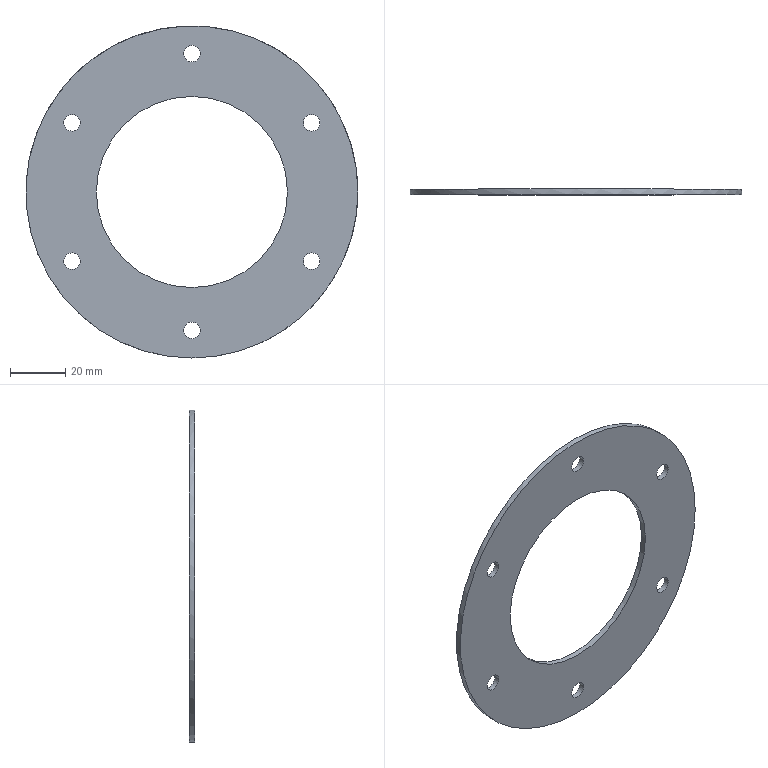Part | NX | features DATUM_CSYS 12, SKETCH 11, HOLE PACKAGE 9, SIMPLE HOLE 9, EXTRACT_DATUM_AXIS 6, EXTRACT_FACE 6, Instance Feature 5, EXTRUDE 4, BLEND 2, DELETE FACE 1, Pattern Feature 1, REPLACE_FACE 1, SWP104 1 | 1 solid | 10 faces | box 120 x 2 x 120 mm | volume 14781 mm3 | cylinder 8 | plane 2 | commonest cylinder face diameters 6 x6 69.097 x1 120 x1
STEP:
#1=CARTESIAN_POINT('',(0.,-9.6,-34.549));
#2=VERTEX_POINT('',#1);
#3=CARTESIAN_POINT('',(0.,-9.6,0.));
#4=DIRECTION('',(0.,-1.,0.));
#5=DIRECTION('',(0.,0.,-1.));
#6=AXIS2_PLACEMENT_3D('',#3,#4,#5);
#7=CIRCLE('',#6,34.549);
#8=EDGE_CURVE('',#2,#2,#7,.F.);
#9=ORIENTED_EDGE('',*,*,#8,.T.);
#10=EDGE_LOOP('',(#9));
#11=FACE_BOUND('',#10,.T.);
#12=CARTESIAN_POINT('',(60.,-9.6,0.));
#13=VERTEX_POINT('',#12);
#14=CARTESIAN_POINT('',(0.,-9.6,0.));
#15=DIRECTION('',(0.,-1.,0.));
#16=DIRECTION('',(1.,0.,0.));
#17=AXIS2_PLACEMENT_3D('',#14,#15,#16);
#18=CIRCLE('',#17,60.);
#19=EDGE_CURVE('',#13,#13,#18,.T.);
#20=ORIENTED_EDGE('',*,*,#19,.T.);
#21=EDGE_LOOP('',(#20));
#22=FACE_BOUND('',#21,.T.);
#23=CARTESIAN_POINT('',(0.,-9.6,53.));
#24=VERTEX_POINT('',#23);
#25=CARTESIAN_POINT('',(0.,-9.6,50.));
#26=DIRECTION('',(0.,1.,0.));
#27=DIRECTION('',(0.,0.,1.));
#28=AXIS2_PLACEMENT_3D('',#25,#26,#27);
#29=CIRCLE('',#28,3.);
#30=EDGE_CURVE('',#24,#24,#29,.T.);
#31=ORIENTED_EDGE('',*,*,#30,.T.);
#32=EDGE_LOOP('',(#31));
#33=FACE_BOUND('',#32,.T.);
#34=CARTESIAN_POINT('',(43.301,-9.6,28.));
#35=VERTEX_POINT('',#34);
#36=CARTESIAN_POINT('',(43.301,-9.6,25.));
#37=DIRECTION('',(0.,1.,0.));
#38=DIRECTION('',(0.,0.,1.));
#39=AXIS2_PLACEMENT_3D('',#36,#37,#38);
#40=CIRCLE('',#39,3.);
#41=EDGE_CURVE('',#35,#35,#40,.T.);
#42=ORIENTED_EDGE('',*,*,#41,.T.);
#43=EDGE_LOOP('',(#42));
#44=FACE_BOUND('',#43,.T.);
#45=CARTESIAN_POINT('',(43.301,-9.6,-22.));
#46=VERTEX_POINT('',#45);
#47=CARTESIAN_POINT('',(43.301,-9.6,-25.));
#48=DIRECTION('',(0.,1.,0.));
#49=DIRECTION('',(0.,0.,1.));
#50=AXIS2_PLACEMENT_3D('',#47,#48,#49);
#51=CIRCLE('',#50,3.);
#52=EDGE_CURVE('',#46,#46,#51,.T.);
#53=ORIENTED_EDGE('',*,*,#52,.T.);
#54=EDGE_LOOP('',(#53));
#55=FACE_BOUND('',#54,.T.);
#56=CARTESIAN_POINT('',(0.,-9.6,-47.));
#57=VERTEX_POINT('',#56);
#58=CARTESIAN_POINT('',(0.,-9.6,-50.));
#59=DIRECTION('',(0.,1.,0.));
#60=DIRECTION('',(0.,0.,1.));
#61=AXIS2_PLACEMENT_3D('',#58,#59,#60);
#62=CIRCLE('',#61,3.);
#63=EDGE_CURVE('',#57,#57,#62,.T.);
#64=ORIENTED_EDGE('',*,*,#63,.T.);
#65=EDGE_LOOP('',(#64));
#66=FACE_BOUND('',#65,.T.);
#67=CARTESIAN_POINT('',(-43.301,-9.6,-22.));
#68=VERTEX_POINT('',#67);
#69=CARTESIAN_POINT('',(-43.301,-9.6,-25.));
#70=DIRECTION('',(0.,1.,0.));
#71=DIRECTION('',(0.,0.,1.));
#72=AXIS2_PLACEMENT_3D('',#69,#70,#71);
#73=CIRCLE('',#72,3.);
#74=EDGE_CURVE('',#68,#68,#73,.T.);
#75=ORIENTED_EDGE('',*,*,#74,.T.);
#76=EDGE_LOOP('',(#75));
#77=FACE_BOUND('',#76,.T.);
#78=CARTESIAN_POINT('',(-43.301,-9.6,28.));
#79=VERTEX_POINT('',#78);
#80=CARTESIAN_POINT('',(-43.301,-9.6,25.));
#81=DIRECTION('',(0.,1.,0.));
#82=DIRECTION('',(0.,0.,1.));
#83=AXIS2_PLACEMENT_3D('',#80,#81,#82);
#84=CIRCLE('',#83,3.);
#85=EDGE_CURVE('',#79,#79,#84,.T.);
#86=ORIENTED_EDGE('',*,*,#85,.T.);
#87=EDGE_LOOP('',(#86));
#88=FACE_BOUND('',#87,.T.);
#89=CARTESIAN_POINT('',(0.,-9.6,0.));
#90=DIRECTION('',(0.,-1.,0.));
#91=DIRECTION('',(0.,0.,-1.));
#92=AXIS2_PLACEMENT_3D('',#89,#90,#91);
#93=PLANE('',#92);
#94=ADVANCED_FACE('',(#11,#22,#33,#44,#55,#66,#77,#88),#93,.T.);
#95=CARTESIAN_POINT('',(0.,-7.6,-60.));
#96=VERTEX_POINT('',#95);
#97=CARTESIAN_POINT('',(0.,-7.6,0.));
#98=DIRECTION('',(0.,-1.,0.));
#99=DIRECTION('',(0.,0.,-1.));
#100=AXIS2_PLACEMENT_3D('',#97,#98,#99);
#101=CIRCLE('',#100,60.);
#102=EDGE_CURVE('',#96,#96,#101,.F.);
#103=ORIENTED_EDGE('',*,*,#102,.F.);
#104=EDGE_LOOP('',(#103));
#105=FACE_BOUND('',#104,.T.);
#106=ORIENTED_EDGE('',*,*,#19,.F.);
#107=EDGE_LOOP('',(#106));
#108=FACE_BOUND('',#107,.T.);
#109=CARTESIAN_POINT('',(0.,0.,0.));
#110=DIRECTION('',(0.,-1.,0.));
#111=DIRECTION('',(0.,0.,-1.));
#112=AXIS2_PLACEMENT_3D('',#109,#110,#111);
#113=CYLINDRICAL_SURFACE('',#112,60.);
#114=ADVANCED_FACE('',(#105,#108),#113,.T.);
#115=CARTESIAN_POINT('',(0.,-7.6,47.));
#116=VERTEX_POINT('',#115);
#117=CARTESIAN_POINT('',(0.,-7.6,50.));
#118=DIRECTION('',(0.,-1.,0.));
#119=DIRECTION('',(0.,0.,-1.));
#120=AXIS2_PLACEMENT_3D('',#117,#118,#119);
#121=CIRCLE('',#120,3.);
#122=EDGE_CURVE('',#116,#116,#121,.F.);
#123=ORIENTED_EDGE('',*,*,#122,.T.);
#124=EDGE_LOOP('',(#123));
#125=FACE_BOUND('',#124,.T.);
#126=ORIENTED_EDGE('',*,*,#30,.F.);
#127=EDGE_LOOP('',(#126));
#128=FACE_BOUND('',#127,.T.);
#129=CARTESIAN_POINT('',(0.,-9.6,50.));
#130=DIRECTION('',(0.,1.,0.));
#131=DIRECTION('',(0.,0.,1.));
#132=AXIS2_PLACEMENT_3D('',#129,#130,#131);
#133=CYLINDRICAL_SURFACE('',#132,3.);
#134=ADVANCED_FACE('',(#125,#128),#133,.F.);
#135=CARTESIAN_POINT('',(43.301,-7.6,22.));
#136=VERTEX_POINT('',#135);
#137=CARTESIAN_POINT('',(43.301,-7.6,25.));
#138=DIRECTION('',(0.,-1.,0.));
#139=DIRECTION('',(0.,0.,-1.));
#140=AXIS2_PLACEMENT_3D('',#137,#138,#139);
#141=CIRCLE('',#140,3.);
#142=EDGE_CURVE('',#136,#136,#141,.F.);
#143=ORIENTED_EDGE('',*,*,#142,.T.);
#144=EDGE_LOOP('',(#143));
#145=FACE_BOUND('',#144,.T.);
#146=ORIENTED_EDGE('',*,*,#41,.F.);
#147=EDGE_LOOP('',(#146));
#148=FACE_BOUND('',#147,.T.);
#149=CARTESIAN_POINT('',(43.301,-9.6,25.));
#150=DIRECTION('',(0.,1.,0.));
#151=DIRECTION('',(0.,0.,1.));
#152=AXIS2_PLACEMENT_3D('',#149,#150,#151);
#153=CYLINDRICAL_SURFACE('',#152,3.);
#154=ADVANCED_FACE('',(#145,#148),#153,.F.);
#155=CARTESIAN_POINT('',(43.301,-7.6,-28.));
#156=VERTEX_POINT('',#155);
#157=CARTESIAN_POINT('',(43.301,-7.6,-25.));
#158=DIRECTION('',(0.,-1.,0.));
#159=DIRECTION('',(0.,0.,-1.));
#160=AXIS2_PLACEMENT_3D('',#157,#158,#159);
#161=CIRCLE('',#160,3.);
#162=EDGE_CURVE('',#156,#156,#161,.F.);
#163=ORIENTED_EDGE('',*,*,#162,.T.);
#164=EDGE_LOOP('',(#163));
#165=FACE_BOUND('',#164,.T.);
#166=ORIENTED_EDGE('',*,*,#52,.F.);
#167=EDGE_LOOP('',(#166));
#168=FACE_BOUND('',#167,.T.);
#169=CARTESIAN_POINT('',(43.301,-9.6,-25.));
#170=DIRECTION('',(0.,1.,0.));
#171=DIRECTION('',(0.,0.,1.));
#172=AXIS2_PLACEMENT_3D('',#169,#170,#171);
#173=CYLINDRICAL_SURFACE('',#172,3.);
#174=ADVANCED_FACE('',(#165,#168),#173,.F.);
#175=CARTESIAN_POINT('',(0.,-7.6,-53.));
#176=VERTEX_POINT('',#175);
#177=CARTESIAN_POINT('',(0.,-7.6,-50.));
#178=DIRECTION('',(0.,-1.,0.));
#179=DIRECTION('',(0.,0.,-1.));
#180=AXIS2_PLACEMENT_3D('',#177,#178,#179);
#181=CIRCLE('',#180,3.);
#182=EDGE_CURVE('',#176,#176,#181,.F.);
#183=ORIENTED_EDGE('',*,*,#182,.T.);
#184=EDGE_LOOP('',(#183));
#185=FACE_BOUND('',#184,.T.);
#186=ORIENTED_EDGE('',*,*,#63,.F.);
#187=EDGE_LOOP('',(#186));
#188=FACE_BOUND('',#187,.T.);
#189=CARTESIAN_POINT('',(0.,-9.6,-50.));
#190=DIRECTION('',(0.,1.,0.));
#191=DIRECTION('',(0.,0.,1.));
#192=AXIS2_PLACEMENT_3D('',#189,#190,#191);
#193=CYLINDRICAL_SURFACE('',#192,3.);
#194=ADVANCED_FACE('',(#185,#188),#193,.F.);
#195=CARTESIAN_POINT('',(-43.301,-7.6,-28.));
#196=VERTEX_POINT('',#195);
#197=CARTESIAN_POINT('',(-43.301,-7.6,-25.));
#198=DIRECTION('',(0.,-1.,0.));
#199=DIRECTION('',(0.,0.,-1.));
#200=AXIS2_PLACEMENT_3D('',#197,#198,#199);
#201=CIRCLE('',#200,3.);
#202=EDGE_CURVE('',#196,#196,#201,.F.);
#203=ORIENTED_EDGE('',*,*,#202,.T.);
#204=EDGE_LOOP('',(#203));
#205=FACE_BOUND('',#204,.T.);
#206=ORIENTED_EDGE('',*,*,#74,.F.);
#207=EDGE_LOOP('',(#206));
#208=FACE_BOUND('',#207,.T.);
#209=CARTESIAN_POINT('',(-43.301,-9.6,-25.));
#210=DIRECTION('',(0.,1.,0.));
#211=DIRECTION('',(0.,0.,1.));
#212=AXIS2_PLACEMENT_3D('',#209,#210,#211);
#213=CYLINDRICAL_SURFACE('',#212,3.);
#214=ADVANCED_FACE('',(#205,#208),#213,.F.);
#215=CARTESIAN_POINT('',(-43.301,-7.6,22.));
#216=VERTEX_POINT('',#215);
#217=CARTESIAN_POINT('',(-43.301,-7.6,25.));
#218=DIRECTION('',(0.,-1.,0.));
#219=DIRECTION('',(0.,0.,-1.));
#220=AXIS2_PLACEMENT_3D('',#217,#218,#219);
#221=CIRCLE('',#220,3.);
#222=EDGE_CURVE('',#216,#216,#221,.F.);
#223=ORIENTED_EDGE('',*,*,#222,.T.);
#224=EDGE_LOOP('',(#223));
#225=FACE_BOUND('',#224,.T.);
#226=ORIENTED_EDGE('',*,*,#85,.F.);
#227=EDGE_LOOP('',(#226));
#228=FACE_BOUND('',#227,.T.);
#229=CARTESIAN_POINT('',(-43.301,-9.6,25.));
#230=DIRECTION('',(0.,1.,0.));
#231=DIRECTION('',(0.,0.,1.));
#232=AXIS2_PLACEMENT_3D('',#229,#230,#231);
#233=CYLINDRICAL_SURFACE('',#232,3.);
#234=ADVANCED_FACE('',(#225,#228),#233,.F.);
#235=CARTESIAN_POINT('',(0.,-7.6,-34.549));
#236=VERTEX_POINT('',#235);
#237=CARTESIAN_POINT('',(0.,-7.6,0.));
#238=DIRECTION('',(0.,-1.,0.));
#239=DIRECTION('',(0.,0.,-1.));
#240=AXIS2_PLACEMENT_3D('',#237,#238,#239);
#241=CIRCLE('',#240,34.549);
#242=EDGE_CURVE('',#236,#236,#241,.F.);
#243=ORIENTED_EDGE('',*,*,#242,.F.);
#244=EDGE_LOOP('',(#243));
#245=FACE_BOUND('',#244,.T.);
#246=ORIENTED_EDGE('',*,*,#122,.F.);
#247=EDGE_LOOP('',(#246));
#248=FACE_BOUND('',#247,.T.);
#249=ORIENTED_EDGE('',*,*,#162,.F.);
#250=EDGE_LOOP('',(#249));
#251=FACE_BOUND('',#250,.T.);
#252=ORIENTED_EDGE('',*,*,#202,.F.);
#253=EDGE_LOOP('',(#252));
#254=FACE_BOUND('',#253,.T.);
#255=ORIENTED_EDGE('',*,*,#222,.F.);
#256=EDGE_LOOP('',(#255));
#257=FACE_BOUND('',#256,.T.);
#258=ORIENTED_EDGE('',*,*,#182,.F.);
#259=EDGE_LOOP('',(#258));
#260=FACE_BOUND('',#259,.T.);
#261=ORIENTED_EDGE('',*,*,#142,.F.);
#262=EDGE_LOOP('',(#261));
#263=FACE_BOUND('',#262,.T.);
#264=ORIENTED_EDGE('',*,*,#102,.T.);
#265=EDGE_LOOP('',(#264));
#266=FACE_BOUND('',#265,.T.);
#267=CARTESIAN_POINT('',(-75.,-7.6,81.));
#268=DIRECTION('',(0.,-1.,0.));
#269=DIRECTION('',(0.,0.,-1.));
#270=AXIS2_PLACEMENT_3D('',#267,#268,#269);
#271=PLANE('',#270);
#272=ADVANCED_FACE('',(#245,#248,#251,#254,#257,#260,#263,#266),#271,.F.);
#273=ORIENTED_EDGE('',*,*,#8,.F.);
#274=EDGE_LOOP('',(#273));
#275=FACE_BOUND('',#274,.T.);
#276=ORIENTED_EDGE('',*,*,#242,.T.);
#277=EDGE_LOOP('',(#276));
#278=FACE_BOUND('',#277,.T.);
#279=CARTESIAN_POINT('',(0.,-61.,0.));
#280=DIRECTION('',(0.,1.,0.));
#281=DIRECTION('',(0.,0.,1.));
#282=AXIS2_PLACEMENT_3D('',#279,#280,#281);
#283=CYLINDRICAL_SURFACE('',#282,34.549);
#284=ADVANCED_FACE('',(#275,#278),#283,.F.);
#285=CLOSED_SHELL('',(#94,#114,#134,#154,#174,#194,#214,#234,#272,#284));
#286=MANIFOLD_SOLID_BREP('',#285);
#287=(LENGTH_UNIT()NAMED_UNIT(*)SI_UNIT(.MILLI.,.METRE.));
#288=UNCERTAINTY_MEASURE_WITH_UNIT(LENGTH_MEASURE(0.00001),#287,'','');
#289=(NAMED_UNIT(*)PLANE_ANGLE_UNIT()SI_UNIT($,.RADIAN.));
#290=(NAMED_UNIT(*)SI_UNIT($,.STERADIAN.)SOLID_ANGLE_UNIT());
#291=(GEOMETRIC_REPRESENTATION_CONTEXT(3)GLOBAL_UNCERTAINTY_ASSIGNED_CONTEXT((#288))GLOBAL_UNIT_ASSIGNED_CONTEXT((#287,#289,#290))REPRESENTATION_CONTEXT('',''));
#292=ADVANCED_BREP_SHAPE_REPRESENTATION('',(#286),#291);